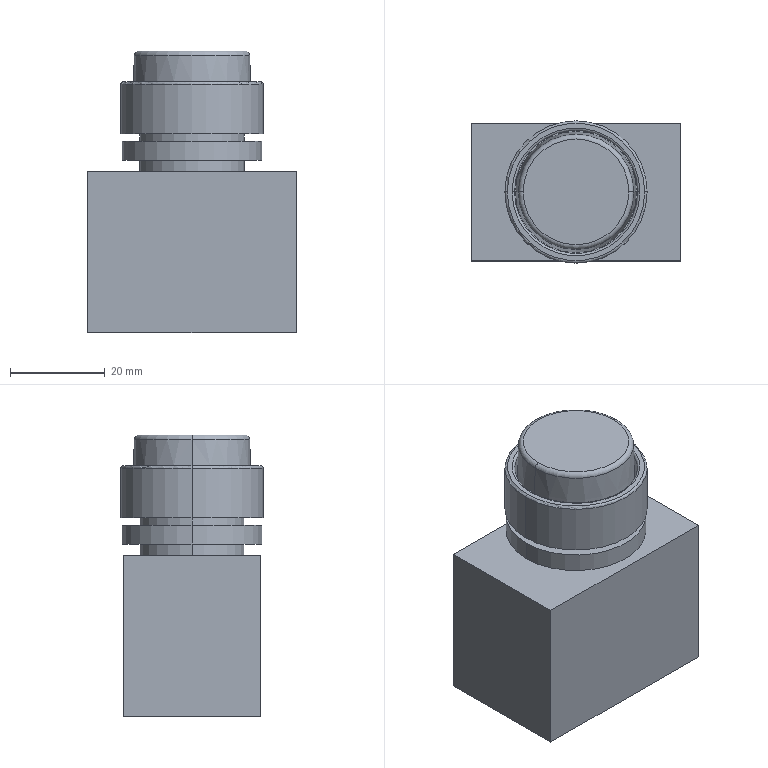Part | SolidWorks | features BaseBody 2 | 2 solids | 30 faces | box 44 x 30 x 59.5 mm | volume 58065 mm3 | plane 12 | cylinder 10 | torus 6 | cone 2 | commonest cylinder face diameters 22 x4 26 x2 29.5 x2 30 x2
STEP:
#1=CARTESIAN_POINT('',(-15.,0.,18.5));
#2=VERTEX_POINT('',#1);
#3=CARTESIAN_POINT('',(15.,0.,18.5));
#4=VERTEX_POINT('',#3);
#5=CARTESIAN_POINT('',(0.,0.,18.5));
#6=DIRECTION('',(0.,0.,-1.));
#7=DIRECTION('',(1.,0.,0.));
#8=AXIS2_PLACEMENT_3D('',#5,#6,#7);
#9=CIRCLE('',#8,15.);
#10=EDGE_CURVE('',#2,#4,#9,.T.);
#11=ORIENTED_EDGE('',*,*,#10,.F.);
#12=CARTESIAN_POINT('',(-14.5,0.,19.));
#13=VERTEX_POINT('',#12);
#14=CARTESIAN_POINT('',(-14.5,0.,18.5));
#15=DIRECTION('',(0.,1.,0.));
#16=DIRECTION('',(-1.,0.,0.));
#17=AXIS2_PLACEMENT_3D('',#14,#15,#16);
#18=CIRCLE('',#17,0.5);
#19=EDGE_CURVE('',#2,#13,#18,.T.);
#20=ORIENTED_EDGE('',*,*,#19,.T.);
#21=CARTESIAN_POINT('',(14.5,0.,19.));
#22=VERTEX_POINT('',#21);
#23=CARTESIAN_POINT('',(0.,0.,19.));
#24=DIRECTION('',(0.,0.,1.));
#25=DIRECTION('',(1.,0.,0.));
#26=AXIS2_PLACEMENT_3D('',#23,#24,#25);
#27=CIRCLE('',#26,14.5);
#28=EDGE_CURVE('',#22,#13,#27,.T.);
#29=ORIENTED_EDGE('',*,*,#28,.F.);
#30=CARTESIAN_POINT('',(14.5,0.,18.5));
#31=DIRECTION('',(0.,-1.,0.));
#32=DIRECTION('',(0.,0.,-1.));
#33=AXIS2_PLACEMENT_3D('',#30,#31,#32);
#34=CIRCLE('',#33,0.5);
#35=EDGE_CURVE('',#4,#22,#34,.T.);
#36=ORIENTED_EDGE('',*,*,#35,.F.);
#37=EDGE_LOOP('',(#11,#20,#29,#36));
#38=FACE_OUTER_BOUND('',#37,.T.);
#39=CARTESIAN_POINT('',(0.,0.,18.5));
#40=DIRECTION('',(0.,0.,1.));
#41=DIRECTION('',(1.,0.,0.));
#42=AXIS2_PLACEMENT_3D('',#39,#40,#41);
#43=TOROIDAL_SURFACE('',#42,14.5,0.5);
#44=ADVANCED_FACE('',(#38),#43,.T.);
#45=CARTESIAN_POINT('',(-13.5,0.,19.));
#46=VERTEX_POINT('',#45);
#47=CARTESIAN_POINT('',(13.5,0.,19.));
#48=VERTEX_POINT('',#47);
#49=CARTESIAN_POINT('',(0.,0.,19.));
#50=DIRECTION('',(0.,0.,-1.));
#51=DIRECTION('',(1.,0.,0.));
#52=AXIS2_PLACEMENT_3D('',#49,#50,#51);
#53=CIRCLE('',#52,13.5);
#54=EDGE_CURVE('',#46,#48,#53,.T.);
#55=ORIENTED_EDGE('',*,*,#54,.F.);
#56=CARTESIAN_POINT('',(-13.,0.,18.5));
#57=VERTEX_POINT('',#56);
#58=CARTESIAN_POINT('',(-13.5,0.,18.5));
#59=DIRECTION('',(0.,1.,0.));
#60=DIRECTION('',(-1.,0.,0.));
#61=AXIS2_PLACEMENT_3D('',#58,#59,#60);
#62=CIRCLE('',#61,0.5);
#63=EDGE_CURVE('',#46,#57,#62,.T.);
#64=ORIENTED_EDGE('',*,*,#63,.T.);
#65=CARTESIAN_POINT('',(13.,0.,18.5));
#66=VERTEX_POINT('',#65);
#67=CARTESIAN_POINT('',(0.,0.,18.5));
#68=DIRECTION('',(0.,0.,1.));
#69=DIRECTION('',(1.,0.,0.));
#70=AXIS2_PLACEMENT_3D('',#67,#68,#69);
#71=CIRCLE('',#70,13.);
#72=EDGE_CURVE('',#66,#57,#71,.T.);
#73=ORIENTED_EDGE('',*,*,#72,.F.);
#74=CARTESIAN_POINT('',(13.5,0.,18.5));
#75=DIRECTION('',(0.,-1.,0.));
#76=DIRECTION('',(0.,0.,-1.));
#77=AXIS2_PLACEMENT_3D('',#74,#75,#76);
#78=CIRCLE('',#77,0.5);
#79=EDGE_CURVE('',#48,#66,#78,.T.);
#80=ORIENTED_EDGE('',*,*,#79,.F.);
#81=EDGE_LOOP('',(#55,#64,#73,#80));
#82=FACE_OUTER_BOUND('',#81,.T.);
#83=CARTESIAN_POINT('',(0.,0.,18.5));
#84=DIRECTION('',(0.,0.,1.));
#85=DIRECTION('',(1.,0.,0.));
#86=AXIS2_PLACEMENT_3D('',#83,#84,#85);
#87=TOROIDAL_SURFACE('',#86,13.5,0.5);
#88=ADVANCED_FACE('',(#82),#87,.T.);
#89=CARTESIAN_POINT('',(0.,0.,18.5));
#90=DIRECTION('',(0.,0.,1.));
#91=DIRECTION('',(1.,0.,0.));
#92=AXIS2_PLACEMENT_3D('',#89,#90,#91);
#93=CIRCLE('',#92,13.);
#94=EDGE_CURVE('',#57,#66,#93,.T.);
#95=ORIENTED_EDGE('',*,*,#94,.T.);
#96=CARTESIAN_POINT('',(13.,0.,8.));
#97=VERTEX_POINT('',#96);
#98=CARTESIAN_POINT('',(13.,0.,19.));
#99=DIRECTION('',(0.,0.,-1.));
#100=VECTOR('',#99,1000.);
#101=LINE('',#98,#100);
#102=EDGE_CURVE('',#66,#97,#101,.T.);
#103=ORIENTED_EDGE('',*,*,#102,.T.);
#104=CARTESIAN_POINT('',(-13.,0.,8.));
#105=VERTEX_POINT('',#104);
#106=CARTESIAN_POINT('',(0.,0.,8.));
#107=DIRECTION('',(0.,0.,1.));
#108=DIRECTION('',(1.,0.,0.));
#109=AXIS2_PLACEMENT_3D('',#106,#107,#108);
#110=CIRCLE('',#109,13.);
#111=EDGE_CURVE('',#105,#97,#110,.T.);
#112=ORIENTED_EDGE('',*,*,#111,.F.);
#113=CARTESIAN_POINT('',(-13.,0.,19.));
#114=DIRECTION('',(0.,0.,-1.));
#115=VECTOR('',#114,1000.);
#116=LINE('',#113,#115);
#117=EDGE_CURVE('',#57,#105,#116,.T.);
#118=ORIENTED_EDGE('',*,*,#117,.F.);
#119=EDGE_LOOP('',(#95,#103,#112,#118));
#120=FACE_OUTER_BOUND('',#119,.T.);
#121=CARTESIAN_POINT('',(0.,0.,19.));
#122=DIRECTION('',(0.,0.,-1.));
#123=DIRECTION('',(-1.,0.,0.));
#124=AXIS2_PLACEMENT_3D('',#121,#122,#123);
#125=CYLINDRICAL_SURFACE('',#124,13.);
#126=ADVANCED_FACE('',(#120),#125,.F.);
#127=ORIENTED_EDGE('',*,*,#10,.T.);
#128=CARTESIAN_POINT('',(15.,0.,8.));
#129=VERTEX_POINT('',#128);
#130=CARTESIAN_POINT('',(15.,0.,19.));
#131=DIRECTION('',(0.,0.,-1.));
#132=VECTOR('',#131,1000.);
#133=LINE('',#130,#132);
#134=EDGE_CURVE('',#4,#129,#133,.T.);
#135=ORIENTED_EDGE('',*,*,#134,.T.);
#136=CARTESIAN_POINT('',(-15.,0.,8.));
#137=VERTEX_POINT('',#136);
#138=CARTESIAN_POINT('',(0.,0.,8.));
#139=DIRECTION('',(0.,0.,1.));
#140=DIRECTION('',(1.,0.,0.));
#141=AXIS2_PLACEMENT_3D('',#138,#139,#140);
#142=CIRCLE('',#141,15.);
#143=EDGE_CURVE('',#129,#137,#142,.T.);
#144=ORIENTED_EDGE('',*,*,#143,.T.);
#145=CARTESIAN_POINT('',(-15.,0.,19.));
#146=DIRECTION('',(0.,0.,-1.));
#147=VECTOR('',#146,1000.);
#148=LINE('',#145,#147);
#149=EDGE_CURVE('',#2,#137,#148,.T.);
#150=ORIENTED_EDGE('',*,*,#149,.F.);
#151=EDGE_LOOP('',(#127,#135,#144,#150));
#152=FACE_OUTER_BOUND('',#151,.T.);
#153=CARTESIAN_POINT('',(0.,0.,19.));
#154=DIRECTION('',(0.,0.,-1.));
#155=DIRECTION('',(-1.,0.,0.));
#156=AXIS2_PLACEMENT_3D('',#153,#154,#155);
#157=CYLINDRICAL_SURFACE('',#156,15.);
#158=ADVANCED_FACE('',(#152),#157,.T.);
#159=CARTESIAN_POINT('',(0.,0.,19.));
#160=DIRECTION('',(0.,0.,-1.));
#161=DIRECTION('',(1.,0.,0.));
#162=AXIS2_PLACEMENT_3D('',#159,#160,#161);
#163=CIRCLE('',#162,13.5);
#164=EDGE_CURVE('',#48,#46,#163,.T.);
#165=ORIENTED_EDGE('',*,*,#164,.T.);
#166=ORIENTED_EDGE('',*,*,#54,.T.);
#167=EDGE_LOOP('',(#165,#166));
#168=FACE_BOUND('',#167,.T.);
#169=ORIENTED_EDGE('',*,*,#28,.T.);
#170=CARTESIAN_POINT('',(0.,0.,19.));
#171=DIRECTION('',(0.,0.,1.));
#172=DIRECTION('',(1.,0.,0.));
#173=AXIS2_PLACEMENT_3D('',#170,#171,#172);
#174=CIRCLE('',#173,14.5);
#175=EDGE_CURVE('',#13,#22,#174,.T.);
#176=ORIENTED_EDGE('',*,*,#175,.T.);
#177=EDGE_LOOP('',(#169,#176));
#178=FACE_OUTER_BOUND('',#177,.T.);
#179=CARTESIAN_POINT('',(0.,0.,19.));
#180=DIRECTION('',(0.,0.,1.));
#181=DIRECTION('',(1.,0.,0.));
#182=AXIS2_PLACEMENT_3D('',#179,#180,#181);
#183=PLANE('',#182);
#184=ADVANCED_FACE('',(#168,#178),#183,.T.);
#185=CARTESIAN_POINT('',(0.,0.,8.));
#186=DIRECTION('',(0.,0.,1.));
#187=DIRECTION('',(1.,0.,0.));
#188=AXIS2_PLACEMENT_3D('',#185,#186,#187);
#189=CIRCLE('',#188,15.);
#190=EDGE_CURVE('',#137,#129,#189,.T.);
#191=ORIENTED_EDGE('',*,*,#190,.F.);
#192=ORIENTED_EDGE('',*,*,#143,.F.);
#193=EDGE_LOOP('',(#191,#192));
#194=FACE_OUTER_BOUND('',#193,.T.);
#195=ORIENTED_EDGE('',*,*,#111,.T.);
#196=CARTESIAN_POINT('',(0.,0.,8.));
#197=DIRECTION('',(0.,0.,1.));
#198=DIRECTION('',(1.,0.,0.));
#199=AXIS2_PLACEMENT_3D('',#196,#197,#198);
#200=CIRCLE('',#199,13.);
#201=EDGE_CURVE('',#97,#105,#200,.T.);
#202=ORIENTED_EDGE('',*,*,#201,.T.);
#203=EDGE_LOOP('',(#195,#202));
#204=FACE_BOUND('',#203,.T.);
#205=CARTESIAN_POINT('',(0.,0.,8.));
#206=DIRECTION('',(0.,0.,1.));
#207=DIRECTION('',(1.,0.,0.));
#208=AXIS2_PLACEMENT_3D('',#205,#206,#207);
#209=PLANE('',#208);
#210=ADVANCED_FACE('',(#194,#204),#209,.F.);
#211=ORIENTED_EDGE('',*,*,#134,.F.);
#212=CARTESIAN_POINT('',(0.,0.,18.5));
#213=DIRECTION('',(0.,0.,-1.));
#214=DIRECTION('',(1.,0.,0.));
#215=AXIS2_PLACEMENT_3D('',#212,#213,#214);
#216=CIRCLE('',#215,15.);
#217=EDGE_CURVE('',#4,#2,#216,.T.);
#218=ORIENTED_EDGE('',*,*,#217,.T.);
#219=ORIENTED_EDGE('',*,*,#149,.T.);
#220=ORIENTED_EDGE('',*,*,#190,.T.);
#221=EDGE_LOOP('',(#211,#218,#219,#220));
#222=FACE_OUTER_BOUND('',#221,.T.);
#223=CARTESIAN_POINT('',(0.,0.,19.));
#224=DIRECTION('',(0.,0.,-1.));
#225=DIRECTION('',(-1.,0.,0.));
#226=AXIS2_PLACEMENT_3D('',#223,#224,#225);
#227=CYLINDRICAL_SURFACE('',#226,15.);
#228=ADVANCED_FACE('',(#222),#227,.T.);
#229=ORIENTED_EDGE('',*,*,#102,.F.);
#230=ORIENTED_EDGE('',*,*,#72,.T.);
#231=ORIENTED_EDGE('',*,*,#117,.T.);
#232=ORIENTED_EDGE('',*,*,#201,.F.);
#233=EDGE_LOOP('',(#229,#230,#231,#232));
#234=FACE_OUTER_BOUND('',#233,.T.);
#235=CARTESIAN_POINT('',(0.,0.,19.));
#236=DIRECTION('',(0.,0.,-1.));
#237=DIRECTION('',(-1.,0.,0.));
#238=AXIS2_PLACEMENT_3D('',#235,#236,#237);
#239=CYLINDRICAL_SURFACE('',#238,13.);
#240=ADVANCED_FACE('',(#234),#239,.F.);
#241=ORIENTED_EDGE('',*,*,#63,.F.);
#242=ORIENTED_EDGE('',*,*,#164,.F.);
#243=ORIENTED_EDGE('',*,*,#79,.T.);
#244=ORIENTED_EDGE('',*,*,#94,.F.);
#245=EDGE_LOOP('',(#241,#242,#243,#244));
#246=FACE_OUTER_BOUND('',#245,.T.);
#247=CARTESIAN_POINT('',(0.,0.,18.5));
#248=DIRECTION('',(0.,0.,1.));
#249=DIRECTION('',(1.,0.,0.));
#250=AXIS2_PLACEMENT_3D('',#247,#248,#249);
#251=TOROIDAL_SURFACE('',#250,13.5,0.5);
#252=ADVANCED_FACE('',(#246),#251,.T.);
#253=ORIENTED_EDGE('',*,*,#19,.F.);
#254=ORIENTED_EDGE('',*,*,#217,.F.);
#255=ORIENTED_EDGE('',*,*,#35,.T.);
#256=ORIENTED_EDGE('',*,*,#175,.F.);
#257=EDGE_LOOP('',(#253,#254,#255,#256));
#258=FACE_OUTER_BOUND('',#257,.T.);
#259=CARTESIAN_POINT('',(0.,0.,18.5));
#260=DIRECTION('',(0.,0.,1.));
#261=DIRECTION('',(1.,0.,0.));
#262=AXIS2_PLACEMENT_3D('',#259,#260,#261);
#263=TOROIDAL_SURFACE('',#262,14.5,0.5);
#264=ADVANCED_FACE('',(#258),#263,.T.);
#265=CLOSED_SHELL('',(#44,#88,#126,#158,#184,#210,#228,#240,#252,#264));
#266=MANIFOLD_SOLID_BREP('',#265);
#267=CARTESIAN_POINT('',(-12.173,0.,24.535));
#268=VERTEX_POINT('',#267);
#269=CARTESIAN_POINT('',(12.173,0.,24.535));
#270=VERTEX_POINT('',#269);
#271=CARTESIAN_POINT('',(0.,0.,24.535));
#272=DIRECTION('',(0.,0.,-1.));
#273=DIRECTION('',(-1.,0.,0.));
#274=AXIS2_PLACEMENT_3D('',#271,#272,#273);
#275=CIRCLE('',#274,12.173);
#276=EDGE_CURVE('',#268,#270,#275,.T.);
#277=ORIENTED_EDGE('',*,*,#276,.F.);
#278=CARTESIAN_POINT('',(-11.173,0.,25.5));
#279=VERTEX_POINT('',#278);
#280=CARTESIAN_POINT('',(-11.173,0.,24.5));
#281=DIRECTION('',(0.,1.,0.));
#282=DIRECTION('',(-1.,0.,0.));
#283=AXIS2_PLACEMENT_3D('',#280,#281,#282);
#284=CIRCLE('',#283,1.);
#285=EDGE_CURVE('',#268,#279,#284,.T.);
#286=ORIENTED_EDGE('',*,*,#285,.T.);
#287=CARTESIAN_POINT('',(11.173,0.,25.5));
#288=VERTEX_POINT('',#287);
#289=CARTESIAN_POINT('',(0.,0.,25.5));
#290=DIRECTION('',(0.,0.,1.));
#291=DIRECTION('',(1.,0.,0.));
#292=AXIS2_PLACEMENT_3D('',#289,#290,#291);
#293=CIRCLE('',#292,11.173);
#294=EDGE_CURVE('',#288,#279,#293,.T.);
#295=ORIENTED_EDGE('',*,*,#294,.F.);
#296=CARTESIAN_POINT('',(11.173,0.,24.5));
#297=DIRECTION('',(0.,-1.,0.));
#298=DIRECTION('',(0.,0.,-1.));
#299=AXIS2_PLACEMENT_3D('',#296,#297,#298);
#300=CIRCLE('',#299,1.);
#301=EDGE_CURVE('',#270,#288,#300,.T.);
#302=ORIENTED_EDGE('',*,*,#301,.F.);
#303=EDGE_LOOP('',(#277,#286,#295,#302));
#304=FACE_OUTER_BOUND('',#303,.T.);
#305=CARTESIAN_POINT('',(0.,0.,24.5));
#306=DIRECTION('',(0.,0.,1.));
#307=DIRECTION('',(1.,0.,0.));
#308=AXIS2_PLACEMENT_3D('',#305,#306,#307);
#309=TOROIDAL_SURFACE('',#308,11.173,1.);
#310=ADVANCED_FACE('',(#304),#309,.T.);
#311=CARTESIAN_POINT('',(0.,0.,24.535));
#312=DIRECTION('',(0.,0.,-1.));
#313=DIRECTION('',(-1.,0.,0.));
#314=AXIS2_PLACEMENT_3D('',#311,#312,#313);
#315=CIRCLE('',#314,12.173);
#316=EDGE_CURVE('',#270,#268,#315,.T.);
#317=ORIENTED_EDGE('',*,*,#316,.T.);
#318=CARTESIAN_POINT('',(-12.75,0.,8.));
#319=VERTEX_POINT('',#318);
#320=CARTESIAN_POINT('',(-12.75,0.,8.));
#321=DIRECTION('',(-0.0349,0.,-0.9994));
#322=VECTOR('',#321,1000.);
#323=LINE('',#320,#322);
#324=EDGE_CURVE('',#268,#319,#323,.T.);
#325=ORIENTED_EDGE('',*,*,#324,.T.);
#326=CARTESIAN_POINT('',(12.75,0.,8.));
#327=VERTEX_POINT('',#326);
#328=CARTESIAN_POINT('',(0.,0.,8.));
#329=DIRECTION('',(0.,0.,1.));
#330=DIRECTION('',(1.,0.,0.));
#331=AXIS2_PLACEMENT_3D('',#328,#329,#330);
#332=CIRCLE('',#331,12.75);
#333=EDGE_CURVE('',#319,#327,#332,.T.);
#334=ORIENTED_EDGE('',*,*,#333,.T.);
#335=CARTESIAN_POINT('',(12.75,0.,8.));
#336=DIRECTION('',(0.0349,0.,-0.9994));
#337=VECTOR('',#336,1000.);
#338=LINE('',#335,#337);
#339=EDGE_CURVE('',#270,#327,#338,.T.);
#340=ORIENTED_EDGE('',*,*,#339,.F.);
#341=EDGE_LOOP('',(#317,#325,#334,#340));
#342=FACE_OUTER_BOUND('',#341,.T.);
#343=CARTESIAN_POINT('',(0.,0.,8.));
#344=DIRECTION('',(0.,0.,-1.));
#345=DIRECTION('',(1.,0.,0.));
#346=AXIS2_PLACEMENT_3D('',#343,#344,#345);
#347=CONICAL_SURFACE('',#346,12.75,0.03491);
#348=ADVANCED_FACE('',(#342),#347,.T.);
#349=CARTESIAN_POINT('',(11.,0.,8.));
#350=VERTEX_POINT('',#349);
#351=CARTESIAN_POINT('',(-11.,0.,8.));
#352=VERTEX_POINT('',#351);
#353=CARTESIAN_POINT('',(0.,0.,8.));
#354=DIRECTION('',(0.,0.,1.));
#355=DIRECTION('',(1.,0.,0.));
#356=AXIS2_PLACEMENT_3D('',#353,#354,#355);
#357=CIRCLE('',#356,11.);
#358=EDGE_CURVE('',#350,#352,#357,.T.);
#359=ORIENTED_EDGE('',*,*,#358,.F.);
#360=CARTESIAN_POINT('',(11.,0.,6.5));
#361=VERTEX_POINT('',#360);
#362=CARTESIAN_POINT('',(11.,0.,8.));
#363=DIRECTION('',(0.,0.,-1.));
#364=VECTOR('',#363,1000.);
#365=LINE('',#362,#364);
#366=EDGE_CURVE('',#350,#361,#365,.T.);
#367=ORIENTED_EDGE('',*,*,#366,.T.);
#368=CARTESIAN_POINT('',(-11.,0.,6.5));
#369=VERTEX_POINT('',#368);
#370=CARTESIAN_POINT('',(0.,0.,6.5));
#371=DIRECTION('',(0.,0.,1.));
#372=DIRECTION('',(1.,0.,0.));
#373=AXIS2_PLACEMENT_3D('',#370,#371,#372);
#374=CIRCLE('',#373,11.);
#375=EDGE_CURVE('',#361,#369,#374,.T.);
#376=ORIENTED_EDGE('',*,*,#375,.T.);
#377=CARTESIAN_POINT('',(-11.,0.,8.));
#378=DIRECTION('',(0.,0.,-1.));
#379=VECTOR('',#378,1000.);
#380=LINE('',#377,#379);
#381=EDGE_CURVE('',#352,#369,#380,.T.);
#382=ORIENTED_EDGE('',*,*,#381,.F.);
#383=EDGE_LOOP('',(#359,#367,#376,#382));
#384=FACE_OUTER_BOUND('',#383,.T.);
#385=CARTESIAN_POINT('',(0.,0.,8.));
#386=DIRECTION('',(0.,0.,-1.));
#387=DIRECTION('',(-1.,0.,0.));
#388=AXIS2_PLACEMENT_3D('',#385,#386,#387);
#389=CYLINDRICAL_SURFACE('',#388,11.);
#390=ADVANCED_FACE('',(#384),#389,.T.);
#391=CARTESIAN_POINT('',(14.75,0.,2.5));
#392=VERTEX_POINT('',#391);
#393=CARTESIAN_POINT('',(-14.75,0.,2.5));
#394=VERTEX_POINT('',#393);
#395=CARTESIAN_POINT('',(0.,0.,2.5));
#396=DIRECTION('',(0.,0.,1.));
#397=DIRECTION('',(1.,0.,0.));
#398=AXIS2_PLACEMENT_3D('',#395,#396,#397);
#399=CIRCLE('',#398,14.75);
#400=EDGE_CURVE('',#392,#394,#399,.T.);
#401=ORIENTED_EDGE('',*,*,#400,.T.);
#402=CARTESIAN_POINT('',(-14.75,0.,6.5));
#403=VERTEX_POINT('',#402);
#404=CARTESIAN_POINT('',(-14.75,0.,2.5));
#405=DIRECTION('',(0.,0.,1.));
#406=VECTOR('',#405,1000.);
#407=LINE('',#404,#406);
#408=EDGE_CURVE('',#394,#403,#407,.T.);
#409=ORIENTED_EDGE('',*,*,#408,.T.);
#410=CARTESIAN_POINT('',(14.75,0.,6.5));
#411=VERTEX_POINT('',#410);
#412=CARTESIAN_POINT('',(0.,0.,6.5));
#413=DIRECTION('',(0.,0.,1.));
#414=DIRECTION('',(1.,0.,0.));
#415=AXIS2_PLACEMENT_3D('',#412,#413,#414);
#416=CIRCLE('',#415,14.75);
#417=EDGE_CURVE('',#411,#403,#416,.T.);
#418=ORIENTED_EDGE('',*,*,#417,.F.);
#419=CARTESIAN_POINT('',(14.75,0.,2.5));
#420=DIRECTION('',(0.,0.,1.));
#421=VECTOR('',#420,1000.);
#422=LINE('',#419,#421);
#423=EDGE_CURVE('',#392,#411,#422,.T.);
#424=ORIENTED_EDGE('',*,*,#423,.F.);
#425=EDGE_LOOP('',(#401,#409,#418,#424));
#426=FACE_OUTER_BOUND('',#425,.T.);
#427=CARTESIAN_POINT('',(0.,0.,2.5));
#428=DIRECTION('',(0.,0.,1.));
#429=DIRECTION('',(1.,0.,0.));
#430=AXIS2_PLACEMENT_3D('',#427,#428,#429);
#431=CYLINDRICAL_SURFACE('',#430,14.75);
#432=ADVANCED_FACE('',(#426),#431,.T.);
#433=CARTESIAN_POINT('',(11.,0.,2.5));
#434=VERTEX_POINT('',#433);
#435=CARTESIAN_POINT('',(-11.,0.,2.5));
#436=VERTEX_POINT('',#435);
#437=CARTESIAN_POINT('',(0.,0.,2.5));
#438=DIRECTION('',(0.,0.,1.));
#439=DIRECTION('',(1.,0.,0.));
#440=AXIS2_PLACEMENT_3D('',#437,#438,#439);
#441=CIRCLE('',#440,11.);
#442=EDGE_CURVE('',#434,#436,#441,.T.);
#443=ORIENTED_EDGE('',*,*,#442,.F.);
#444=CARTESIAN_POINT('',(11.,0.,0.));
#445=VERTEX_POINT('',#444);
#446=CARTESIAN_POINT('',(11.,0.,8.));
#447=DIRECTION('',(0.,0.,-1.));
#448=VECTOR('',#447,1000.);
#449=LINE('',#446,#448);
#450=EDGE_CURVE('',#434,#445,#449,.T.);
#451=ORIENTED_EDGE('',*,*,#450,.T.);
#452=CARTESIAN_POINT('',(-11.,0.,0.));
#453=VERTEX_POINT('',#452);
#454=CARTESIAN_POINT('',(0.,0.,0.));
#455=DIRECTION('',(0.,0.,1.));
#456=DIRECTION('',(1.,0.,0.));
#457=AXIS2_PLACEMENT_3D('',#454,#455,#456);
#458=CIRCLE('',#457,11.);
#459=EDGE_CURVE('',#445,#453,#458,.T.);
#460=ORIENTED_EDGE('',*,*,#459,.T.);
#461=CARTESIAN_POINT('',(-11.,0.,8.));
#462=DIRECTION('',(0.,0.,-1.));
#463=VECTOR('',#462,1000.);
#464=LINE('',#461,#463);
#465=EDGE_CURVE('',#436,#453,#464,.T.);
#466=ORIENTED_EDGE('',*,*,#465,.F.);
#467=EDGE_LOOP('',(#443,#451,#460,#466));
#468=FACE_OUTER_BOUND('',#467,.T.);
#469=CARTESIAN_POINT('',(0.,0.,8.));
#470=DIRECTION('',(0.,0.,-1.));
#471=DIRECTION('',(-1.,0.,0.));
#472=AXIS2_PLACEMENT_3D('',#469,#470,#471);
#473=CYLINDRICAL_SURFACE('',#472,11.);
#474=ADVANCED_FACE('',(#468),#473,.T.);
#475=ORIENTED_EDGE('',*,*,#450,.F.);
#476=CARTESIAN_POINT('',(0.,0.,2.5));
#477=DIRECTION('',(0.,0.,1.));
#478=DIRECTION('',(1.,0.,0.));
#479=AXIS2_PLACEMENT_3D('',#476,#477,#478);
#480=CIRCLE('',#479,11.);
#481=EDGE_CURVE('',#436,#434,#480,.T.);
#482=ORIENTED_EDGE('',*,*,#481,.F.);
#483=ORIENTED_EDGE('',*,*,#465,.T.);
#484=CARTESIAN_POINT('',(0.,0.,0.));
#485=DIRECTION('',(0.,0.,1.));
#486=DIRECTION('',(1.,0.,0.));
#487=AXIS2_PLACEMENT_3D('',#484,#485,#486);
#488=CIRCLE('',#487,11.);
#489=EDGE_CURVE('',#453,#445,#488,.T.);
#490=ORIENTED_EDGE('',*,*,#489,.T.);
#491=EDGE_LOOP('',(#475,#482,#483,#490));
#492=FACE_OUTER_BOUND('',#491,.T.);
#493=CARTESIAN_POINT('',(0.,0.,8.));
#494=DIRECTION('',(0.,0.,-1.));
#495=DIRECTION('',(-1.,0.,0.));
#496=AXIS2_PLACEMENT_3D('',#493,#494,#495);
#497=CYLINDRICAL_SURFACE('',#496,11.);
#498=ADVANCED_FACE('',(#492),#497,.T.);
#499=CARTESIAN_POINT('',(-22.,14.5,0.));
#500=VERTEX_POINT('',#499);
#501=CARTESIAN_POINT('',(-22.,-14.5,0.));
#502=VERTEX_POINT('',#501);
#503=CARTESIAN_POINT('',(-22.,14.5,0.));
#504=DIRECTION('',(0.,-1.,0.));
#505=VECTOR('',#504,1000.);
#506=LINE('',#503,#505);
#507=EDGE_CURVE('',#500,#502,#506,.T.);
#508=ORIENTED_EDGE('',*,*,#507,.T.);
#509=CARTESIAN_POINT('',(22.,-14.5,0.));
#510=VERTEX_POINT('',#509);
#511=CARTESIAN_POINT('',(-22.,-14.5,0.));
#512=DIRECTION('',(1.,0.,0.));
#513=VECTOR('',#512,1000.);
#514=LINE('',#511,#513);
#515=EDGE_CURVE('',#502,#510,#514,.T.);
#516=ORIENTED_EDGE('',*,*,#515,.T.);
#517=CARTESIAN_POINT('',(22.,14.5,0.));
#518=VERTEX_POINT('',#517);
#519=CARTESIAN_POINT('',(22.,14.5,0.));
#520=DIRECTION('',(0.,1.,0.));
#521=VECTOR('',#520,1000.);
#522=LINE('',#519,#521);
#523=EDGE_CURVE('',#510,#518,#522,.T.);
#524=ORIENTED_EDGE('',*,*,#523,.T.);
#525=CARTESIAN_POINT('',(-22.,14.5,0.));
#526=DIRECTION('',(-1.,0.,0.));
#527=VECTOR('',#526,1000.);
#528=LINE('',#525,#527);
#529=EDGE_CURVE('',#518,#500,#528,.T.);
#530=ORIENTED_EDGE('',*,*,#529,.T.);
#531=EDGE_LOOP('',(#508,#516,#524,#530));
#532=FACE_OUTER_BOUND('',#531,.T.);
#533=ORIENTED_EDGE('',*,*,#489,.F.);
#534=ORIENTED_EDGE('',*,*,#459,.F.);
#535=EDGE_LOOP('',(#533,#534));
#536=FACE_BOUND('',#535,.T.);
#537=CARTESIAN_POINT('',(-22.,-14.5,0.));
#538=DIRECTION('',(0.,0.,1.));
#539=DIRECTION('',(1.,0.,0.));
#540=AXIS2_PLACEMENT_3D('',#537,#538,#539);
#541=PLANE('',#540);
#542=ADVANCED_FACE('',(#532,#536),#541,.T.);
#543=ORIENTED_EDGE('',*,*,#507,.F.);
#544=CARTESIAN_POINT('',(-22.,14.5,-34.));
#545=VERTEX_POINT('',#544);
#546=CARTESIAN_POINT('',(-22.,14.5,-34.));
#547=DIRECTION('',(0.,0.,1.));
#548=VECTOR('',#547,1000.);
#549=LINE('',#546,#548);
#550=EDGE_CURVE('',#545,#500,#549,.T.);
#551=ORIENTED_EDGE('',*,*,#550,.F.);
#552=CARTESIAN_POINT('',(-22.,-14.5,-34.));
#553=VERTEX_POINT('',#552);
#554=CARTESIAN_POINT('',(-22.,14.5,-34.));
#555=DIRECTION('',(0.,-1.,0.));
#556=VECTOR('',#555,1000.);
#557=LINE('',#554,#556);
#558=EDGE_CURVE('',#545,#553,#557,.T.);
#559=ORIENTED_EDGE('',*,*,#558,.T.);
#560=CARTESIAN_POINT('',(-22.,-14.5,-34.));
#561=DIRECTION('',(0.,0.,1.));
#562=VECTOR('',#561,1000.);
#563=LINE('',#560,#562);
#564=EDGE_CURVE('',#553,#502,#563,.T.);
#565=ORIENTED_EDGE('',*,*,#564,.T.);
#566=EDGE_LOOP('',(#543,#551,#559,#565));
#567=FACE_OUTER_BOUND('',#566,.T.);
#568=CARTESIAN_POINT('',(-22.,14.5,-34.));
#569=DIRECTION('',(-1.,0.,0.));
#570=DIRECTION('',(0.,-1.,0.));
#571=AXIS2_PLACEMENT_3D('',#568,#569,#570);
#572=PLANE('',#571);
#573=ADVANCED_FACE('',(#567),#572,.T.);
#574=ORIENTED_EDGE('',*,*,#529,.F.);
#575=CARTESIAN_POINT('',(22.,14.5,-34.));
#576=VERTEX_POINT('',#575);
#577=CARTESIAN_POINT('',(22.,14.5,-34.));
#578=DIRECTION('',(0.,0.,1.));
#579=VECTOR('',#578,1000.);
#580=LINE('',#577,#579);
#581=EDGE_CURVE('',#576,#518,#580,.T.);
#582=ORIENTED_EDGE('',*,*,#581,.F.);
#583=CARTESIAN_POINT('',(-22.,14.5,-34.));
#584=DIRECTION('',(-1.,0.,0.));
#585=VECTOR('',#584,1000.);
#586=LINE('',#583,#585);
#587=EDGE_CURVE('',#576,#545,#586,.T.);
#588=ORIENTED_EDGE('',*,*,#587,.T.);
#589=ORIENTED_EDGE('',*,*,#550,.T.);
#590=EDGE_LOOP('',(#574,#582,#588,#589));
#591=FACE_OUTER_BOUND('',#590,.T.);
#592=CARTESIAN_POINT('',(-22.,14.5,-34.));
#593=DIRECTION('',(0.,1.,0.));
#594=DIRECTION('',(0.,0.,1.));
#595=AXIS2_PLACEMENT_3D('',#592,#593,#594);
#596=PLANE('',#595);
#597=ADVANCED_FACE('',(#591),#596,.T.);
#598=ORIENTED_EDGE('',*,*,#523,.F.);
#599=CARTESIAN_POINT('',(22.,-14.5,-34.));
#600=VERTEX_POINT('',#599);
#601=CARTESIAN_POINT('',(22.,-14.5,-34.));
#602=DIRECTION('',(0.,0.,1.));
#603=VECTOR('',#602,1000.);
#604=LINE('',#601,#603);
#605=EDGE_CURVE('',#600,#510,#604,.T.);
#606=ORIENTED_EDGE('',*,*,#605,.F.);
#607=CARTESIAN_POINT('',(22.,14.5,-34.));
#608=DIRECTION('',(0.,1.,0.));
#609=VECTOR('',#608,1000.);
#610=LINE('',#607,#609);
#611=EDGE_CURVE('',#600,#576,#610,.T.);
#612=ORIENTED_EDGE('',*,*,#611,.T.);
#613=ORIENTED_EDGE('',*,*,#581,.T.);
#614=EDGE_LOOP('',(#598,#606,#612,#613));
#615=FACE_OUTER_BOUND('',#614,.T.);
#616=CARTESIAN_POINT('',(22.,14.5,-34.));
#617=DIRECTION('',(1.,0.,0.));
#618=DIRECTION('',(0.,1.,0.));
#619=AXIS2_PLACEMENT_3D('',#616,#617,#618);
#620=PLANE('',#619);
#621=ADVANCED_FACE('',(#615),#620,.T.);
#622=ORIENTED_EDGE('',*,*,#515,.F.);
#623=ORIENTED_EDGE('',*,*,#564,.F.);
#624=CARTESIAN_POINT('',(-22.,-14.5,-34.));
#625=DIRECTION('',(1.,0.,0.));
#626=VECTOR('',#625,1000.);
#627=LINE('',#624,#626);
#628=EDGE_CURVE('',#553,#600,#627,.T.);
#629=ORIENTED_EDGE('',*,*,#628,.T.);
#630=ORIENTED_EDGE('',*,*,#605,.T.);
#631=EDGE_LOOP('',(#622,#623,#629,#630));
#632=FACE_OUTER_BOUND('',#631,.T.);
#633=CARTESIAN_POINT('',(-22.,-14.5,-34.));
#634=DIRECTION('',(0.,-1.,0.));
#635=DIRECTION('',(1.,0.,0.));
#636=AXIS2_PLACEMENT_3D('',#633,#634,#635);
#637=PLANE('',#636);
#638=ADVANCED_FACE('',(#632),#637,.T.);
#639=ORIENTED_EDGE('',*,*,#558,.F.);
#640=ORIENTED_EDGE('',*,*,#587,.F.);
#641=ORIENTED_EDGE('',*,*,#611,.F.);
#642=ORIENTED_EDGE('',*,*,#628,.F.);
#643=EDGE_LOOP('',(#639,#640,#641,#642));
#644=FACE_OUTER_BOUND('',#643,.T.);
#645=CARTESIAN_POINT('',(-22.,-14.5,-34.));
#646=DIRECTION('',(0.,0.,1.));
#647=DIRECTION('',(1.,0.,0.));
#648=AXIS2_PLACEMENT_3D('',#645,#646,#647);
#649=PLANE('',#648);
#650=ADVANCED_FACE('',(#644),#649,.F.);
#651=ORIENTED_EDGE('',*,*,#400,.F.);
#652=CARTESIAN_POINT('',(0.,0.,2.5));
#653=DIRECTION('',(0.,0.,1.));
#654=DIRECTION('',(1.,0.,0.));
#655=AXIS2_PLACEMENT_3D('',#652,#653,#654);
#656=CIRCLE('',#655,14.75);
#657=EDGE_CURVE('',#394,#392,#656,.T.);
#658=ORIENTED_EDGE('',*,*,#657,.F.);
#659=EDGE_LOOP('',(#651,#658));
#660=FACE_OUTER_BOUND('',#659,.T.);
#661=ORIENTED_EDGE('',*,*,#481,.T.);
#662=ORIENTED_EDGE('',*,*,#442,.T.);
#663=EDGE_LOOP('',(#661,#662));
#664=FACE_BOUND('',#663,.T.);
#665=CARTESIAN_POINT('',(0.,0.,2.5));
#666=DIRECTION('',(0.,0.,1.));
#667=DIRECTION('',(1.,0.,0.));
#668=AXIS2_PLACEMENT_3D('',#665,#666,#667);
#669=PLANE('',#668);
#670=ADVANCED_FACE('',(#660,#664),#669,.F.);
#671=ORIENTED_EDGE('',*,*,#417,.T.);
#672=CARTESIAN_POINT('',(0.,0.,6.5));
#673=DIRECTION('',(0.,0.,1.));
#674=DIRECTION('',(1.,0.,0.));
#675=AXIS2_PLACEMENT_3D('',#672,#673,#674);
#676=CIRCLE('',#675,14.75);
#677=EDGE_CURVE('',#403,#411,#676,.T.);
#678=ORIENTED_EDGE('',*,*,#677,.T.);
#679=EDGE_LOOP('',(#671,#678));
#680=FACE_OUTER_BOUND('',#679,.T.);
#681=CARTESIAN_POINT('',(0.,0.,6.5));
#682=DIRECTION('',(0.,0.,1.));
#683=DIRECTION('',(1.,0.,0.));
#684=AXIS2_PLACEMENT_3D('',#681,#682,#683);
#685=CIRCLE('',#684,11.);
#686=EDGE_CURVE('',#369,#361,#685,.T.);
#687=ORIENTED_EDGE('',*,*,#686,.F.);
#688=ORIENTED_EDGE('',*,*,#375,.F.);
#689=EDGE_LOOP('',(#687,#688));
#690=FACE_BOUND('',#689,.T.);
#691=CARTESIAN_POINT('',(0.,0.,6.5));
#692=DIRECTION('',(0.,0.,1.));
#693=DIRECTION('',(1.,0.,0.));
#694=AXIS2_PLACEMENT_3D('',#691,#692,#693);
#695=PLANE('',#694);
#696=ADVANCED_FACE('',(#680,#690),#695,.T.);
#697=ORIENTED_EDGE('',*,*,#408,.F.);
#698=ORIENTED_EDGE('',*,*,#657,.T.);
#699=ORIENTED_EDGE('',*,*,#423,.T.);
#700=ORIENTED_EDGE('',*,*,#677,.F.);
#701=EDGE_LOOP('',(#697,#698,#699,#700));
#702=FACE_OUTER_BOUND('',#701,.T.);
#703=CARTESIAN_POINT('',(0.,0.,2.5));
#704=DIRECTION('',(0.,0.,1.));
#705=DIRECTION('',(1.,0.,0.));
#706=AXIS2_PLACEMENT_3D('',#703,#704,#705);
#707=CYLINDRICAL_SURFACE('',#706,14.75);
#708=ADVANCED_FACE('',(#702),#707,.T.);
#709=ORIENTED_EDGE('',*,*,#366,.F.);
#710=CARTESIAN_POINT('',(0.,0.,8.));
#711=DIRECTION('',(0.,0.,1.));
#712=DIRECTION('',(1.,0.,0.));
#713=AXIS2_PLACEMENT_3D('',#710,#711,#712);
#714=CIRCLE('',#713,11.);
#715=EDGE_CURVE('',#352,#350,#714,.T.);
#716=ORIENTED_EDGE('',*,*,#715,.F.);
#717=ORIENTED_EDGE('',*,*,#381,.T.);
#718=ORIENTED_EDGE('',*,*,#686,.T.);
#719=EDGE_LOOP('',(#709,#716,#717,#718));
#720=FACE_OUTER_BOUND('',#719,.T.);
#721=CARTESIAN_POINT('',(0.,0.,8.));
#722=DIRECTION('',(0.,0.,-1.));
#723=DIRECTION('',(-1.,0.,0.));
#724=AXIS2_PLACEMENT_3D('',#721,#722,#723);
#725=CYLINDRICAL_SURFACE('',#724,11.);
#726=ADVANCED_FACE('',(#720),#725,.T.);
#727=CARTESIAN_POINT('',(0.,0.,8.));
#728=DIRECTION('',(0.,0.,1.));
#729=DIRECTION('',(1.,0.,0.));
#730=AXIS2_PLACEMENT_3D('',#727,#728,#729);
#731=CIRCLE('',#730,12.75);
#732=EDGE_CURVE('',#327,#319,#731,.T.);
#733=ORIENTED_EDGE('',*,*,#732,.F.);
#734=ORIENTED_EDGE('',*,*,#333,.F.);
#735=EDGE_LOOP('',(#733,#734));
#736=FACE_OUTER_BOUND('',#735,.T.);
#737=ORIENTED_EDGE('',*,*,#715,.T.);
#738=ORIENTED_EDGE('',*,*,#358,.T.);
#739=EDGE_LOOP('',(#737,#738));
#740=FACE_BOUND('',#739,.T.);
#741=CARTESIAN_POINT('',(0.,0.,8.));
#742=DIRECTION('',(0.,0.,1.));
#743=DIRECTION('',(1.,0.,0.));
#744=AXIS2_PLACEMENT_3D('',#741,#742,#743);
#745=PLANE('',#744);
#746=ADVANCED_FACE('',(#736,#740),#745,.F.);
#747=ORIENTED_EDGE('',*,*,#324,.F.);
#748=ORIENTED_EDGE('',*,*,#276,.T.);
#749=ORIENTED_EDGE('',*,*,#339,.T.);
#750=ORIENTED_EDGE('',*,*,#732,.T.);
#751=EDGE_LOOP('',(#747,#748,#749,#750));
#752=FACE_OUTER_BOUND('',#751,.T.);
#753=CARTESIAN_POINT('',(0.,0.,8.));
#754=DIRECTION('',(0.,0.,-1.));
#755=DIRECTION('',(1.,0.,0.));
#756=AXIS2_PLACEMENT_3D('',#753,#754,#755);
#757=CONICAL_SURFACE('',#756,12.75,0.03491);
#758=ADVANCED_FACE('',(#752),#757,.T.);
#759=ORIENTED_EDGE('',*,*,#294,.T.);
#760=CARTESIAN_POINT('',(0.,0.,25.5));
#761=DIRECTION('',(0.,0.,1.));
#762=DIRECTION('',(1.,0.,0.));
#763=AXIS2_PLACEMENT_3D('',#760,#761,#762);
#764=CIRCLE('',#763,11.173);
#765=EDGE_CURVE('',#279,#288,#764,.T.);
#766=ORIENTED_EDGE('',*,*,#765,.T.);
#767=EDGE_LOOP('',(#759,#766));
#768=FACE_OUTER_BOUND('',#767,.T.);
#769=CARTESIAN_POINT('',(0.,0.,25.5));
#770=DIRECTION('',(0.,0.,1.));
#771=DIRECTION('',(1.,0.,0.));
#772=AXIS2_PLACEMENT_3D('',#769,#770,#771);
#773=PLANE('',#772);
#774=ADVANCED_FACE('',(#768),#773,.T.);
#775=ORIENTED_EDGE('',*,*,#285,.F.);
#776=ORIENTED_EDGE('',*,*,#316,.F.);
#777=ORIENTED_EDGE('',*,*,#301,.T.);
#778=ORIENTED_EDGE('',*,*,#765,.F.);
#779=EDGE_LOOP('',(#775,#776,#777,#778));
#780=FACE_OUTER_BOUND('',#779,.T.);
#781=CARTESIAN_POINT('',(0.,0.,24.5));
#782=DIRECTION('',(0.,0.,1.));
#783=DIRECTION('',(1.,0.,0.));
#784=AXIS2_PLACEMENT_3D('',#781,#782,#783);
#785=TOROIDAL_SURFACE('',#784,11.173,1.);
#786=ADVANCED_FACE('',(#780),#785,.T.);
#787=CLOSED_SHELL('',(#310,#348,#390,#432,#474,#498,#542,#573,#597,#621,#638,#650,#670,#696,#708,#726,#746,#758,#774,#786));
#788=MANIFOLD_SOLID_BREP('',#787);
#789=CARTESIAN_POINT('',(0.,0.,0.));
#790=DIRECTION('',(0.,0.,1.));
#791=DIRECTION('',(1.,0.,0.));
#792=AXIS2_PLACEMENT_3D('',#789,#790,#791);
#793=(LENGTH_UNIT()NAMED_UNIT(*)SI_UNIT(.MILLI.,.METRE.));
#794=UNCERTAINTY_MEASURE_WITH_UNIT(LENGTH_MEASURE(0.00001),#793,'','');
#795=(NAMED_UNIT(*)PLANE_ANGLE_UNIT()SI_UNIT($,.RADIAN.));
#796=(NAMED_UNIT(*)SI_UNIT($,.STERADIAN.)SOLID_ANGLE_UNIT());
#797=(GEOMETRIC_REPRESENTATION_CONTEXT(3)GLOBAL_UNCERTAINTY_ASSIGNED_CONTEXT((#794))GLOBAL_UNIT_ASSIGNED_CONTEXT((#793,#795,#796))REPRESENTATION_CONTEXT('',''));
#798=ADVANCED_BREP_SHAPE_REPRESENTATION('',(#266,#788,#792),#797);